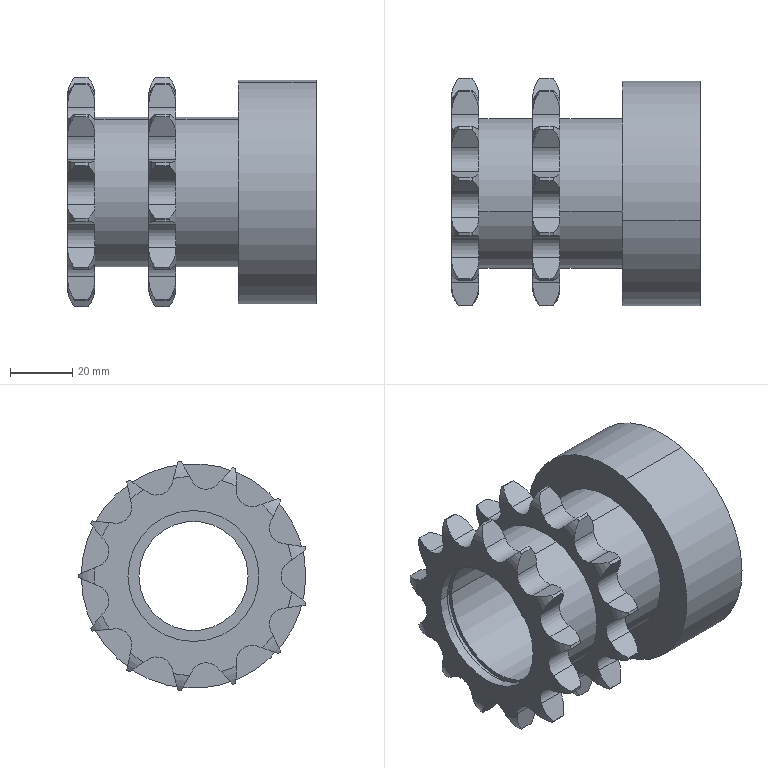Part | STEP file | DCV-000-002 | 1 solid | 181 faces | box 79.7 x 73.041 x 73.574 mm | volume 132681 mm3 | cylinder 68 | plane 61 | torus 52 | commonest cylinder face diameters 74 x28 10.16 x26 42 x4 48 x4 35 x2 44.5 x2